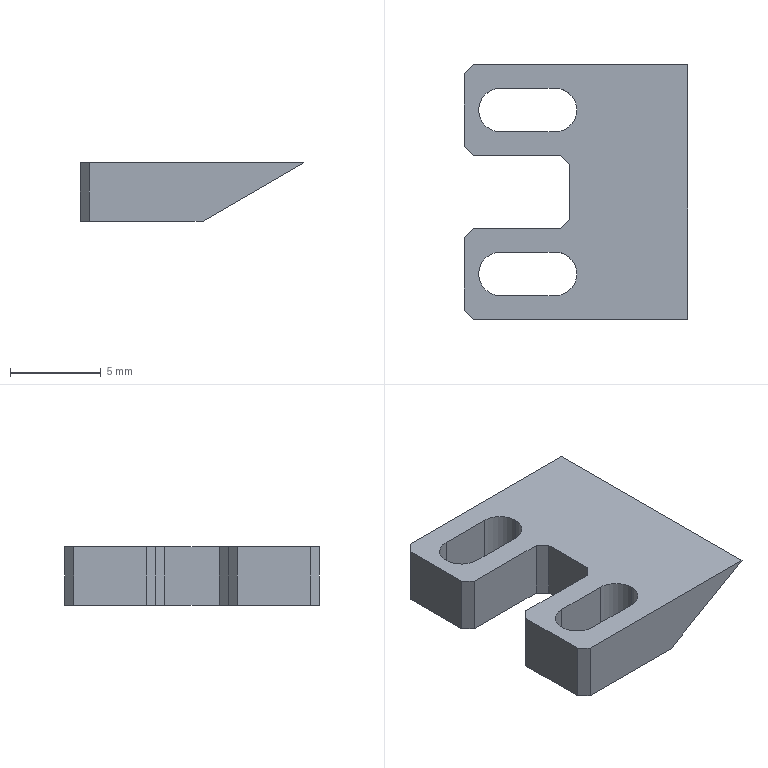Part | NX | 1 solid | 26 faces | box 12.3 x 14 x 3.2 mm | volume 276.814 mm3 | plane 20 | cylinder 6 | commonest cylinder face diameters 2.4 x6
STEP:
#1=CARTESIAN_POINT('',(0.05,4.5,-3.2));
#2=VERTEX_POINT('',#1);
#3=CARTESIAN_POINT('',(-1.15,5.7,-3.2));
#4=VERTEX_POINT('',#3);
#5=CARTESIAN_POINT('',(-1.15,4.5,-3.2));
#6=DIRECTION('',(0.,0.,1.));
#7=DIRECTION('',(1.,0.,0.));
#8=AXIS2_PLACEMENT_3D('',#5,#6,#7);
#9=CIRCLE('',#8,1.2);
#10=EDGE_CURVE('',#2,#4,#9,.T.);
#11=ORIENTED_EDGE('',*,*,#10,.F.);
#12=CARTESIAN_POINT('',(0.05,4.5,0.));
#13=VERTEX_POINT('',#12);
#14=CARTESIAN_POINT('',(0.05,4.5,-3.2));
#15=DIRECTION('',(0.,0.,1.));
#16=VECTOR('',#15,1000.);
#17=LINE('',#14,#16);
#18=EDGE_CURVE('',#2,#13,#17,.T.);
#19=ORIENTED_EDGE('',*,*,#18,.T.);
#20=CARTESIAN_POINT('',(-1.15,5.7,0.));
#21=VERTEX_POINT('',#20);
#22=CARTESIAN_POINT('',(-1.15,4.5,0.));
#23=DIRECTION('',(0.,0.,1.));
#24=DIRECTION('',(1.,0.,0.));
#25=AXIS2_PLACEMENT_3D('',#22,#23,#24);
#26=CIRCLE('',#25,1.2);
#27=EDGE_CURVE('',#13,#21,#26,.T.);
#28=ORIENTED_EDGE('',*,*,#27,.T.);
#29=CARTESIAN_POINT('',(-1.15,5.7,-3.2));
#30=DIRECTION('',(0.,0.,1.));
#31=VECTOR('',#30,1000.);
#32=LINE('',#29,#31);
#33=EDGE_CURVE('',#4,#21,#32,.T.);
#34=ORIENTED_EDGE('',*,*,#33,.F.);
#35=EDGE_LOOP('',(#11,#19,#28,#34));
#36=FACE_BOUND('',#35,.T.);
#37=CARTESIAN_POINT('',(-1.15,4.5,-3.2));
#38=DIRECTION('',(0.,0.,1.));
#39=DIRECTION('',(-1.,0.,0.));
#40=AXIS2_PLACEMENT_3D('',#37,#38,#39);
#41=CYLINDRICAL_SURFACE('',#40,1.2);
#42=ADVANCED_FACE('',(#36),#41,.F.);
#43=CARTESIAN_POINT('',(0.05,-4.5,-3.2));
#44=VERTEX_POINT('',#43);
#45=CARTESIAN_POINT('',(-1.15,-3.3,-3.2));
#46=VERTEX_POINT('',#45);
#47=CARTESIAN_POINT('',(-1.15,-4.5,-3.2));
#48=DIRECTION('',(0.,0.,1.));
#49=DIRECTION('',(-1.,0.,0.));
#50=AXIS2_PLACEMENT_3D('',#47,#48,#49);
#51=CIRCLE('',#50,1.2);
#52=EDGE_CURVE('',#44,#46,#51,.T.);
#53=ORIENTED_EDGE('',*,*,#52,.F.);
#54=CARTESIAN_POINT('',(0.05,-4.5,0.));
#55=VERTEX_POINT('',#54);
#56=CARTESIAN_POINT('',(0.05,-4.5,-3.2));
#57=DIRECTION('',(0.,0.,1.));
#58=VECTOR('',#57,1000.);
#59=LINE('',#56,#58);
#60=EDGE_CURVE('',#44,#55,#59,.T.);
#61=ORIENTED_EDGE('',*,*,#60,.T.);
#62=CARTESIAN_POINT('',(-1.15,-3.3,0.));
#63=VERTEX_POINT('',#62);
#64=CARTESIAN_POINT('',(-1.15,-4.5,0.));
#65=DIRECTION('',(0.,0.,1.));
#66=DIRECTION('',(-1.,0.,0.));
#67=AXIS2_PLACEMENT_3D('',#64,#65,#66);
#68=CIRCLE('',#67,1.2);
#69=EDGE_CURVE('',#55,#63,#68,.T.);
#70=ORIENTED_EDGE('',*,*,#69,.T.);
#71=CARTESIAN_POINT('',(-1.15,-3.3,-3.2));
#72=DIRECTION('',(0.,0.,1.));
#73=VECTOR('',#72,1000.);
#74=LINE('',#71,#73);
#75=EDGE_CURVE('',#46,#63,#74,.T.);
#76=ORIENTED_EDGE('',*,*,#75,.F.);
#77=EDGE_LOOP('',(#53,#61,#70,#76));
#78=FACE_BOUND('',#77,.T.);
#79=CARTESIAN_POINT('',(-1.15,-4.5,-3.2));
#80=DIRECTION('',(0.,0.,1.));
#81=DIRECTION('',(-1.,0.,0.));
#82=AXIS2_PLACEMENT_3D('',#79,#80,#81);
#83=CYLINDRICAL_SURFACE('',#82,1.2);
#84=ADVANCED_FACE('',(#78),#83,.F.);
#85=CARTESIAN_POINT('',(-6.15,6.5,-3.2));
#86=VERTEX_POINT('',#85);
#87=CARTESIAN_POINT('',(-6.15,2.5,-3.2));
#88=VERTEX_POINT('',#87);
#89=CARTESIAN_POINT('',(-6.15,7.,-3.2));
#90=DIRECTION('',(0.,-1.,0.));
#91=VECTOR('',#90,1000.);
#92=LINE('',#89,#91);
#93=EDGE_CURVE('',#86,#88,#92,.T.);
#94=ORIENTED_EDGE('',*,*,#93,.T.);
#95=CARTESIAN_POINT('',(-6.15,2.5,0.));
#96=VERTEX_POINT('',#95);
#97=CARTESIAN_POINT('',(-6.15,2.5,0.));
#98=DIRECTION('',(0.,0.,1.));
#99=VECTOR('',#98,1000.);
#100=LINE('',#97,#99);
#101=EDGE_CURVE('',#88,#96,#100,.T.);
#102=ORIENTED_EDGE('',*,*,#101,.T.);
#103=CARTESIAN_POINT('',(-6.15,6.5,0.));
#104=VERTEX_POINT('',#103);
#105=CARTESIAN_POINT('',(-6.15,7.,0.));
#106=DIRECTION('',(0.,-1.,0.));
#107=VECTOR('',#106,1000.);
#108=LINE('',#105,#107);
#109=EDGE_CURVE('',#104,#96,#108,.T.);
#110=ORIENTED_EDGE('',*,*,#109,.F.);
#111=CARTESIAN_POINT('',(-6.15,6.5,-3.2));
#112=DIRECTION('',(0.,0.,-1.));
#113=VECTOR('',#112,1000.);
#114=LINE('',#111,#113);
#115=EDGE_CURVE('',#104,#86,#114,.T.);
#116=ORIENTED_EDGE('',*,*,#115,.T.);
#117=EDGE_LOOP('',(#94,#102,#110,#116));
#118=FACE_BOUND('',#117,.T.);
#119=CARTESIAN_POINT('',(-6.15,7.,0.));
#120=DIRECTION('',(1.,0.,0.));
#121=DIRECTION('',(0.,-1.,0.));
#122=AXIS2_PLACEMENT_3D('',#119,#120,#121);
#123=PLANE('',#122);
#124=ADVANCED_FACE('',(#118),#123,.F.);
#125=CARTESIAN_POINT('',(6.15,-7.,0.));
#126=VERTEX_POINT('',#125);
#127=CARTESIAN_POINT('',(0.6074,-7.,-3.2));
#128=VERTEX_POINT('',#127);
#129=CARTESIAN_POINT('',(0.6074,-7.,-3.2));
#130=DIRECTION('',(-0.866,0.,-0.5));
#131=VECTOR('',#130,1000.);
#132=LINE('',#129,#131);
#133=EDGE_CURVE('',#126,#128,#132,.T.);
#134=ORIENTED_EDGE('',*,*,#133,.T.);
#135=CARTESIAN_POINT('',(0.6074,7.,-3.2));
#136=VERTEX_POINT('',#135);
#137=CARTESIAN_POINT('',(0.6074,7.,-3.2));
#138=DIRECTION('',(0.,-1.,0.));
#139=VECTOR('',#138,1000.);
#140=LINE('',#137,#139);
#141=EDGE_CURVE('',#136,#128,#140,.T.);
#142=ORIENTED_EDGE('',*,*,#141,.F.);
#143=CARTESIAN_POINT('',(6.15,7.,0.));
#144=VERTEX_POINT('',#143);
#145=CARTESIAN_POINT('',(0.6074,7.,-3.2));
#146=DIRECTION('',(-0.866,0.,-0.5));
#147=VECTOR('',#146,1000.);
#148=LINE('',#145,#147);
#149=EDGE_CURVE('',#144,#136,#148,.T.);
#150=ORIENTED_EDGE('',*,*,#149,.F.);
#151=CARTESIAN_POINT('',(6.15,7.,0.));
#152=DIRECTION('',(0.,-1.,0.));
#153=VECTOR('',#152,1000.);
#154=LINE('',#151,#153);
#155=EDGE_CURVE('',#144,#126,#154,.T.);
#156=ORIENTED_EDGE('',*,*,#155,.T.);
#157=EDGE_LOOP('',(#134,#142,#150,#156));
#158=FACE_BOUND('',#157,.T.);
#159=CARTESIAN_POINT('',(0.6074,7.,-3.2));
#160=DIRECTION('',(-0.5,0.,0.866));
#161=DIRECTION('',(-0.866,0.,-0.5));
#162=AXIS2_PLACEMENT_3D('',#159,#160,#161);
#163=PLANE('',#162);
#164=ADVANCED_FACE('',(#158),#163,.F.);
#165=CARTESIAN_POINT('',(-4.15,3.3,-3.2));
#166=VERTEX_POINT('',#165);
#167=CARTESIAN_POINT('',(-1.15,3.3,-3.2));
#168=VERTEX_POINT('',#167);
#169=CARTESIAN_POINT('',(-1.15,3.3,-3.2));
#170=DIRECTION('',(1.,0.,0.));
#171=VECTOR('',#170,1000.);
#172=LINE('',#169,#171);
#173=EDGE_CURVE('',#166,#168,#172,.T.);
#174=ORIENTED_EDGE('',*,*,#173,.T.);
#175=CARTESIAN_POINT('',(-1.15,4.5,-3.2));
#176=DIRECTION('',(0.,0.,1.));
#177=DIRECTION('',(1.,0.,0.));
#178=AXIS2_PLACEMENT_3D('',#175,#176,#177);
#179=CIRCLE('',#178,1.2);
#180=EDGE_CURVE('',#168,#2,#179,.T.);
#181=ORIENTED_EDGE('',*,*,#180,.T.);
#182=ORIENTED_EDGE('',*,*,#10,.T.);
#183=CARTESIAN_POINT('',(-4.15,5.7,-3.2));
#184=VERTEX_POINT('',#183);
#185=CARTESIAN_POINT('',(-1.15,5.7,-3.2));
#186=DIRECTION('',(-1.,0.,0.));
#187=VECTOR('',#186,1000.);
#188=LINE('',#185,#187);
#189=EDGE_CURVE('',#4,#184,#188,.T.);
#190=ORIENTED_EDGE('',*,*,#189,.T.);
#191=CARTESIAN_POINT('',(-4.15,4.5,-3.2));
#192=DIRECTION('',(0.,0.,1.));
#193=DIRECTION('',(1.,0.,0.));
#194=AXIS2_PLACEMENT_3D('',#191,#192,#193);
#195=CIRCLE('',#194,1.2);
#196=EDGE_CURVE('',#184,#166,#195,.T.);
#197=ORIENTED_EDGE('',*,*,#196,.T.);
#198=EDGE_LOOP('',(#174,#181,#182,#190,#197));
#199=FACE_BOUND('',#198,.T.);
#200=CARTESIAN_POINT('',(-4.15,-5.7,-3.2));
#201=VERTEX_POINT('',#200);
#202=CARTESIAN_POINT('',(-1.15,-5.7,-3.2));
#203=VERTEX_POINT('',#202);
#204=CARTESIAN_POINT('',(-1.15,-5.7,-3.2));
#205=DIRECTION('',(1.,0.,0.));
#206=VECTOR('',#205,1000.);
#207=LINE('',#204,#206);
#208=EDGE_CURVE('',#201,#203,#207,.T.);
#209=ORIENTED_EDGE('',*,*,#208,.T.);
#210=CARTESIAN_POINT('',(-1.15,-4.5,-3.2));
#211=DIRECTION('',(0.,0.,1.));
#212=DIRECTION('',(-1.,0.,0.));
#213=AXIS2_PLACEMENT_3D('',#210,#211,#212);
#214=CIRCLE('',#213,1.2);
#215=EDGE_CURVE('',#203,#44,#214,.T.);
#216=ORIENTED_EDGE('',*,*,#215,.T.);
#217=ORIENTED_EDGE('',*,*,#52,.T.);
#218=CARTESIAN_POINT('',(-4.15,-3.3,-3.2));
#219=VERTEX_POINT('',#218);
#220=CARTESIAN_POINT('',(-1.15,-3.3,-3.2));
#221=DIRECTION('',(-1.,0.,0.));
#222=VECTOR('',#221,1000.);
#223=LINE('',#220,#222);
#224=EDGE_CURVE('',#46,#219,#223,.T.);
#225=ORIENTED_EDGE('',*,*,#224,.T.);
#226=CARTESIAN_POINT('',(-4.15,-4.5,-3.2));
#227=DIRECTION('',(0.,0.,1.));
#228=DIRECTION('',(-1.,0.,0.));
#229=AXIS2_PLACEMENT_3D('',#226,#227,#228);
#230=CIRCLE('',#229,1.2);
#231=EDGE_CURVE('',#219,#201,#230,.T.);
#232=ORIENTED_EDGE('',*,*,#231,.T.);
#233=EDGE_LOOP('',(#209,#216,#217,#225,#232));
#234=FACE_BOUND('',#233,.T.);
#235=CARTESIAN_POINT('',(-5.65,-7.,-3.2));
#236=VERTEX_POINT('',#235);
#237=CARTESIAN_POINT('',(-6.15,-7.,-3.2));
#238=DIRECTION('',(-1.,0.,0.));
#239=VECTOR('',#238,1000.);
#240=LINE('',#237,#239);
#241=EDGE_CURVE('',#128,#236,#240,.T.);
#242=ORIENTED_EDGE('',*,*,#241,.T.);
#243=CARTESIAN_POINT('',(-6.15,-6.5,-3.2));
#244=VERTEX_POINT('',#243);
#245=CARTESIAN_POINT('',(-6.15,-6.5,-3.2));
#246=DIRECTION('',(-0.7071,0.7071,0.));
#247=VECTOR('',#246,1000.);
#248=LINE('',#245,#247);
#249=EDGE_CURVE('',#236,#244,#248,.T.);
#250=ORIENTED_EDGE('',*,*,#249,.T.);
#251=CARTESIAN_POINT('',(-6.15,-2.5,-3.2));
#252=VERTEX_POINT('',#251);
#253=CARTESIAN_POINT('',(-6.15,7.,-3.2));
#254=DIRECTION('',(0.,-1.,0.));
#255=VECTOR('',#254,1000.);
#256=LINE('',#253,#255);
#257=EDGE_CURVE('',#252,#244,#256,.T.);
#258=ORIENTED_EDGE('',*,*,#257,.F.);
#259=CARTESIAN_POINT('',(-5.65,-2.,-3.2));
#260=VERTEX_POINT('',#259);
#261=CARTESIAN_POINT('',(-5.65,-2.,-3.2));
#262=DIRECTION('',(0.7071,0.7071,0.));
#263=VECTOR('',#262,1000.);
#264=LINE('',#261,#263);
#265=EDGE_CURVE('',#252,#260,#264,.T.);
#266=ORIENTED_EDGE('',*,*,#265,.T.);
#267=CARTESIAN_POINT('',(-0.85,-2.,-3.2));
#268=VERTEX_POINT('',#267);
#269=CARTESIAN_POINT('',(-0.35,-2.,-3.2));
#270=DIRECTION('',(1.,0.,0.));
#271=VECTOR('',#270,1000.);
#272=LINE('',#269,#271);
#273=EDGE_CURVE('',#260,#268,#272,.T.);
#274=ORIENTED_EDGE('',*,*,#273,.T.);
#275=CARTESIAN_POINT('',(-0.35,-1.5,-3.2));
#276=VERTEX_POINT('',#275);
#277=CARTESIAN_POINT('',(1.,-0.15,-3.2));
#278=DIRECTION('',(0.7071,0.7071,0.));
#279=VECTOR('',#278,1000.);
#280=LINE('',#277,#279);
#281=EDGE_CURVE('',#268,#276,#280,.T.);
#282=ORIENTED_EDGE('',*,*,#281,.T.);
#283=CARTESIAN_POINT('',(-0.35,1.5,-3.2));
#284=VERTEX_POINT('',#283);
#285=CARTESIAN_POINT('',(-0.35,2.,-3.2));
#286=DIRECTION('',(0.,1.,0.));
#287=VECTOR('',#286,1000.);
#288=LINE('',#285,#287);
#289=EDGE_CURVE('',#276,#284,#288,.T.);
#290=ORIENTED_EDGE('',*,*,#289,.T.);
#291=CARTESIAN_POINT('',(-0.85,2.,-3.2));
#292=VERTEX_POINT('',#291);
#293=CARTESIAN_POINT('',(-6.,7.15,-3.2));
#294=DIRECTION('',(-0.7071,0.7071,0.));
#295=VECTOR('',#294,1000.);
#296=LINE('',#293,#295);
#297=EDGE_CURVE('',#284,#292,#296,.T.);
#298=ORIENTED_EDGE('',*,*,#297,.T.);
#299=CARTESIAN_POINT('',(-5.65,2.,-3.2));
#300=VERTEX_POINT('',#299);
#301=CARTESIAN_POINT('',(-6.15,2.,-3.2));
#302=DIRECTION('',(-1.,0.,0.));
#303=VECTOR('',#302,1000.);
#304=LINE('',#301,#303);
#305=EDGE_CURVE('',#292,#300,#304,.T.);
#306=ORIENTED_EDGE('',*,*,#305,.T.);
#307=CARTESIAN_POINT('',(-6.15,2.5,-3.2));
#308=DIRECTION('',(-0.7071,0.7071,0.));
#309=VECTOR('',#308,1000.);
#310=LINE('',#307,#309);
#311=EDGE_CURVE('',#300,#88,#310,.T.);
#312=ORIENTED_EDGE('',*,*,#311,.T.);
#313=ORIENTED_EDGE('',*,*,#93,.F.);
#314=CARTESIAN_POINT('',(-5.65,7.,-3.2));
#315=VERTEX_POINT('',#314);
#316=CARTESIAN_POINT('',(-5.65,7.,-3.2));
#317=DIRECTION('',(0.7071,0.7071,0.));
#318=VECTOR('',#317,1000.);
#319=LINE('',#316,#318);
#320=EDGE_CURVE('',#86,#315,#319,.T.);
#321=ORIENTED_EDGE('',*,*,#320,.T.);
#322=CARTESIAN_POINT('',(-6.15,7.,-3.2));
#323=DIRECTION('',(-1.,0.,0.));
#324=VECTOR('',#323,1000.);
#325=LINE('',#322,#324);
#326=EDGE_CURVE('',#136,#315,#325,.T.);
#327=ORIENTED_EDGE('',*,*,#326,.F.);
#328=ORIENTED_EDGE('',*,*,#141,.T.);
#329=EDGE_LOOP('',(#242,#250,#258,#266,#274,#282,#290,#298,#306,#312,#313,#321,#327,#328));
#330=FACE_BOUND('',#329,.T.);
#331=CARTESIAN_POINT('',(-6.15,7.,-3.2));
#332=DIRECTION('',(0.,0.,1.));
#333=DIRECTION('',(0.,1.,0.));
#334=AXIS2_PLACEMENT_3D('',#331,#332,#333);
#335=PLANE('',#334);
#336=ADVANCED_FACE('',(#199,#234,#330),#335,.F.);
#337=ORIENTED_EDGE('',*,*,#257,.T.);
#338=CARTESIAN_POINT('',(-6.15,-6.5,0.));
#339=VERTEX_POINT('',#338);
#340=CARTESIAN_POINT('',(-6.15,-6.5,0.));
#341=DIRECTION('',(0.,0.,1.));
#342=VECTOR('',#341,1000.);
#343=LINE('',#340,#342);
#344=EDGE_CURVE('',#244,#339,#343,.T.);
#345=ORIENTED_EDGE('',*,*,#344,.T.);
#346=CARTESIAN_POINT('',(-6.15,-2.5,0.));
#347=VERTEX_POINT('',#346);
#348=CARTESIAN_POINT('',(-6.15,7.,0.));
#349=DIRECTION('',(0.,-1.,0.));
#350=VECTOR('',#349,1000.);
#351=LINE('',#348,#350);
#352=EDGE_CURVE('',#347,#339,#351,.T.);
#353=ORIENTED_EDGE('',*,*,#352,.F.);
#354=CARTESIAN_POINT('',(-6.15,-2.5,0.));
#355=DIRECTION('',(0.,0.,-1.));
#356=VECTOR('',#355,1000.);
#357=LINE('',#354,#356);
#358=EDGE_CURVE('',#347,#252,#357,.T.);
#359=ORIENTED_EDGE('',*,*,#358,.T.);
#360=EDGE_LOOP('',(#337,#345,#353,#359));
#361=FACE_BOUND('',#360,.T.);
#362=CARTESIAN_POINT('',(-6.15,7.,0.));
#363=DIRECTION('',(1.,0.,0.));
#364=DIRECTION('',(0.,-1.,0.));
#365=AXIS2_PLACEMENT_3D('',#362,#363,#364);
#366=PLANE('',#365);
#367=ADVANCED_FACE('',(#361),#366,.F.);
#368=CARTESIAN_POINT('',(-4.15,5.7,0.));
#369=VERTEX_POINT('',#368);
#370=CARTESIAN_POINT('',(-1.15,5.7,0.));
#371=DIRECTION('',(-1.,0.,0.));
#372=VECTOR('',#371,1000.);
#373=LINE('',#370,#372);
#374=EDGE_CURVE('',#21,#369,#373,.T.);
#375=ORIENTED_EDGE('',*,*,#374,.F.);
#376=ORIENTED_EDGE('',*,*,#27,.F.);
#377=CARTESIAN_POINT('',(-1.15,3.3,0.));
#378=VERTEX_POINT('',#377);
#379=CARTESIAN_POINT('',(-1.15,4.5,0.));
#380=DIRECTION('',(0.,0.,1.));
#381=DIRECTION('',(1.,0.,0.));
#382=AXIS2_PLACEMENT_3D('',#379,#380,#381);
#383=CIRCLE('',#382,1.2);
#384=EDGE_CURVE('',#378,#13,#383,.T.);
#385=ORIENTED_EDGE('',*,*,#384,.F.);
#386=CARTESIAN_POINT('',(-4.15,3.3,0.));
#387=VERTEX_POINT('',#386);
#388=CARTESIAN_POINT('',(-1.15,3.3,0.));
#389=DIRECTION('',(1.,0.,0.));
#390=VECTOR('',#389,1000.);
#391=LINE('',#388,#390);
#392=EDGE_CURVE('',#387,#378,#391,.T.);
#393=ORIENTED_EDGE('',*,*,#392,.F.);
#394=CARTESIAN_POINT('',(-4.15,4.5,0.));
#395=DIRECTION('',(0.,0.,1.));
#396=DIRECTION('',(1.,0.,0.));
#397=AXIS2_PLACEMENT_3D('',#394,#395,#396);
#398=CIRCLE('',#397,1.2);
#399=EDGE_CURVE('',#369,#387,#398,.T.);
#400=ORIENTED_EDGE('',*,*,#399,.F.);
#401=EDGE_LOOP('',(#375,#376,#385,#393,#400));
#402=FACE_BOUND('',#401,.T.);
#403=CARTESIAN_POINT('',(-4.15,-3.3,0.));
#404=VERTEX_POINT('',#403);
#405=CARTESIAN_POINT('',(-1.15,-3.3,0.));
#406=DIRECTION('',(-1.,0.,0.));
#407=VECTOR('',#406,1000.);
#408=LINE('',#405,#407);
#409=EDGE_CURVE('',#63,#404,#408,.T.);
#410=ORIENTED_EDGE('',*,*,#409,.F.);
#411=ORIENTED_EDGE('',*,*,#69,.F.);
#412=CARTESIAN_POINT('',(-1.15,-5.7,0.));
#413=VERTEX_POINT('',#412);
#414=CARTESIAN_POINT('',(-1.15,-4.5,0.));
#415=DIRECTION('',(0.,0.,1.));
#416=DIRECTION('',(-1.,0.,0.));
#417=AXIS2_PLACEMENT_3D('',#414,#415,#416);
#418=CIRCLE('',#417,1.2);
#419=EDGE_CURVE('',#413,#55,#418,.T.);
#420=ORIENTED_EDGE('',*,*,#419,.F.);
#421=CARTESIAN_POINT('',(-4.15,-5.7,0.));
#422=VERTEX_POINT('',#421);
#423=CARTESIAN_POINT('',(-1.15,-5.7,0.));
#424=DIRECTION('',(1.,0.,0.));
#425=VECTOR('',#424,1000.);
#426=LINE('',#423,#425);
#427=EDGE_CURVE('',#422,#413,#426,.T.);
#428=ORIENTED_EDGE('',*,*,#427,.F.);
#429=CARTESIAN_POINT('',(-4.15,-4.5,0.));
#430=DIRECTION('',(0.,0.,1.));
#431=DIRECTION('',(-1.,0.,0.));
#432=AXIS2_PLACEMENT_3D('',#429,#430,#431);
#433=CIRCLE('',#432,1.2);
#434=EDGE_CURVE('',#404,#422,#433,.T.);
#435=ORIENTED_EDGE('',*,*,#434,.F.);
#436=EDGE_LOOP('',(#410,#411,#420,#428,#435));
#437=FACE_BOUND('',#436,.T.);
#438=ORIENTED_EDGE('',*,*,#352,.T.);
#439=CARTESIAN_POINT('',(-5.65,-7.,0.));
#440=VERTEX_POINT('',#439);
#441=CARTESIAN_POINT('',(-6.15,-6.5,0.));
#442=DIRECTION('',(0.7071,-0.7071,0.));
#443=VECTOR('',#442,1000.);
#444=LINE('',#441,#443);
#445=EDGE_CURVE('',#339,#440,#444,.T.);
#446=ORIENTED_EDGE('',*,*,#445,.T.);
#447=CARTESIAN_POINT('',(6.15,-7.,0.));
#448=DIRECTION('',(1.,0.,0.));
#449=VECTOR('',#448,1000.);
#450=LINE('',#447,#449);
#451=EDGE_CURVE('',#440,#126,#450,.T.);
#452=ORIENTED_EDGE('',*,*,#451,.T.);
#453=ORIENTED_EDGE('',*,*,#155,.F.);
#454=CARTESIAN_POINT('',(-5.65,7.,0.));
#455=VERTEX_POINT('',#454);
#456=CARTESIAN_POINT('',(6.15,7.,0.));
#457=DIRECTION('',(1.,0.,0.));
#458=VECTOR('',#457,1000.);
#459=LINE('',#456,#458);
#460=EDGE_CURVE('',#455,#144,#459,.T.);
#461=ORIENTED_EDGE('',*,*,#460,.F.);
#462=CARTESIAN_POINT('',(-5.65,7.,0.));
#463=DIRECTION('',(-0.7071,-0.7071,0.));
#464=VECTOR('',#463,1000.);
#465=LINE('',#462,#464);
#466=EDGE_CURVE('',#455,#104,#465,.T.);
#467=ORIENTED_EDGE('',*,*,#466,.T.);
#468=ORIENTED_EDGE('',*,*,#109,.T.);
#469=CARTESIAN_POINT('',(-5.65,2.,0.));
#470=VERTEX_POINT('',#469);
#471=CARTESIAN_POINT('',(-6.15,2.5,0.));
#472=DIRECTION('',(0.7071,-0.7071,0.));
#473=VECTOR('',#472,1000.);
#474=LINE('',#471,#473);
#475=EDGE_CURVE('',#96,#470,#474,.T.);
#476=ORIENTED_EDGE('',*,*,#475,.T.);
#477=CARTESIAN_POINT('',(-0.85,2.,0.));
#478=VERTEX_POINT('',#477);
#479=CARTESIAN_POINT('',(-6.15,2.,0.));
#480=DIRECTION('',(-1.,0.,0.));
#481=VECTOR('',#480,1000.);
#482=LINE('',#479,#481);
#483=EDGE_CURVE('',#478,#470,#482,.T.);
#484=ORIENTED_EDGE('',*,*,#483,.F.);
#485=CARTESIAN_POINT('',(-0.35,1.5,0.));
#486=VERTEX_POINT('',#485);
#487=CARTESIAN_POINT('',(0.15,1.,0.));
#488=DIRECTION('',(0.7071,-0.7071,0.));
#489=VECTOR('',#488,1000.);
#490=LINE('',#487,#489);
#491=EDGE_CURVE('',#478,#486,#490,.T.);
#492=ORIENTED_EDGE('',*,*,#491,.T.);
#493=CARTESIAN_POINT('',(-0.35,-1.5,0.));
#494=VERTEX_POINT('',#493);
#495=CARTESIAN_POINT('',(-0.35,2.,0.));
#496=DIRECTION('',(0.,1.,0.));
#497=VECTOR('',#496,1000.);
#498=LINE('',#495,#497);
#499=EDGE_CURVE('',#494,#486,#498,.T.);
#500=ORIENTED_EDGE('',*,*,#499,.F.);
#501=CARTESIAN_POINT('',(-0.85,-2.,0.));
#502=VERTEX_POINT('',#501);
#503=CARTESIAN_POINT('',(7.15,6.,0.));
#504=DIRECTION('',(-0.7071,-0.7071,0.));
#505=VECTOR('',#504,1000.);
#506=LINE('',#503,#505);
#507=EDGE_CURVE('',#494,#502,#506,.T.);
#508=ORIENTED_EDGE('',*,*,#507,.T.);
#509=CARTESIAN_POINT('',(-5.65,-2.,0.));
#510=VERTEX_POINT('',#509);
#511=CARTESIAN_POINT('',(-0.35,-2.,0.));
#512=DIRECTION('',(1.,0.,0.));
#513=VECTOR('',#512,1000.);
#514=LINE('',#511,#513);
#515=EDGE_CURVE('',#510,#502,#514,.T.);
#516=ORIENTED_EDGE('',*,*,#515,.F.);
#517=CARTESIAN_POINT('',(-5.65,-2.,0.));
#518=DIRECTION('',(-0.7071,-0.7071,0.));
#519=VECTOR('',#518,1000.);
#520=LINE('',#517,#519);
#521=EDGE_CURVE('',#510,#347,#520,.T.);
#522=ORIENTED_EDGE('',*,*,#521,.T.);
#523=EDGE_LOOP('',(#438,#446,#452,#453,#461,#467,#468,#476,#484,#492,#500,#508,#516,#522));
#524=FACE_BOUND('',#523,.T.);
#525=CARTESIAN_POINT('',(6.15,7.,0.));
#526=DIRECTION('',(0.,0.,-1.));
#527=DIRECTION('',(1.,0.,0.));
#528=AXIS2_PLACEMENT_3D('',#525,#526,#527);
#529=PLANE('',#528);
#530=ADVANCED_FACE('',(#402,#437,#524),#529,.F.);
#531=ORIENTED_EDGE('',*,*,#326,.T.);
#532=CARTESIAN_POINT('',(-5.65,7.,0.));
#533=DIRECTION('',(0.,0.,1.));
#534=VECTOR('',#533,1000.);
#535=LINE('',#532,#534);
#536=EDGE_CURVE('',#315,#455,#535,.T.);
#537=ORIENTED_EDGE('',*,*,#536,.T.);
#538=ORIENTED_EDGE('',*,*,#460,.T.);
#539=ORIENTED_EDGE('',*,*,#149,.T.);
#540=EDGE_LOOP('',(#531,#537,#538,#539));
#541=FACE_BOUND('',#540,.T.);
#542=CARTESIAN_POINT('',(6.15,7.,0.));
#543=DIRECTION('',(0.,1.,0.));
#544=DIRECTION('',(0.,0.,-1.));
#545=AXIS2_PLACEMENT_3D('',#542,#543,#544);
#546=PLANE('',#545);
#547=ADVANCED_FACE('',(#541),#546,.T.);
#548=ORIENTED_EDGE('',*,*,#451,.F.);
#549=CARTESIAN_POINT('',(-5.65,-7.,0.));
#550=DIRECTION('',(0.,0.,-1.));
#551=VECTOR('',#550,1000.);
#552=LINE('',#549,#551);
#553=EDGE_CURVE('',#440,#236,#552,.T.);
#554=ORIENTED_EDGE('',*,*,#553,.T.);
#555=ORIENTED_EDGE('',*,*,#241,.F.);
#556=ORIENTED_EDGE('',*,*,#133,.F.);
#557=EDGE_LOOP('',(#548,#554,#555,#556));
#558=FACE_BOUND('',#557,.T.);
#559=CARTESIAN_POINT('',(6.15,-7.,0.));
#560=DIRECTION('',(0.,1.,0.));
#561=DIRECTION('',(0.,0.,-1.));
#562=AXIS2_PLACEMENT_3D('',#559,#560,#561);
#563=PLANE('',#562);
#564=ADVANCED_FACE('',(#558),#563,.F.);
#565=ORIENTED_EDGE('',*,*,#305,.F.);
#566=CARTESIAN_POINT('',(-0.85,2.,0.));
#567=DIRECTION('',(0.,0.,1.));
#568=VECTOR('',#567,1000.);
#569=LINE('',#566,#568);
#570=EDGE_CURVE('',#292,#478,#569,.T.);
#571=ORIENTED_EDGE('',*,*,#570,.T.);
#572=ORIENTED_EDGE('',*,*,#483,.T.);
#573=CARTESIAN_POINT('',(-5.65,2.,-3.2));
#574=DIRECTION('',(0.,0.,-1.));
#575=VECTOR('',#574,1000.);
#576=LINE('',#573,#575);
#577=EDGE_CURVE('',#470,#300,#576,.T.);
#578=ORIENTED_EDGE('',*,*,#577,.T.);
#579=EDGE_LOOP('',(#565,#571,#572,#578));
#580=FACE_BOUND('',#579,.T.);
#581=CARTESIAN_POINT('',(-6.15,2.,-3.2));
#582=DIRECTION('',(0.,1.,0.));
#583=DIRECTION('',(0.,0.,-1.));
#584=AXIS2_PLACEMENT_3D('',#581,#582,#583);
#585=PLANE('',#584);
#586=ADVANCED_FACE('',(#580),#585,.F.);
#587=ORIENTED_EDGE('',*,*,#289,.F.);
#588=CARTESIAN_POINT('',(-0.35,-1.5,0.));
#589=DIRECTION('',(0.,0.,1.));
#590=VECTOR('',#589,1000.);
#591=LINE('',#588,#590);
#592=EDGE_CURVE('',#276,#494,#591,.T.);
#593=ORIENTED_EDGE('',*,*,#592,.T.);
#594=ORIENTED_EDGE('',*,*,#499,.T.);
#595=CARTESIAN_POINT('',(-0.35,1.5,-3.2));
#596=DIRECTION('',(0.,0.,-1.));
#597=VECTOR('',#596,1000.);
#598=LINE('',#595,#597);
#599=EDGE_CURVE('',#486,#284,#598,.T.);
#600=ORIENTED_EDGE('',*,*,#599,.T.);
#601=EDGE_LOOP('',(#587,#593,#594,#600));
#602=FACE_BOUND('',#601,.T.);
#603=CARTESIAN_POINT('',(-0.35,2.,-3.2));
#604=DIRECTION('',(1.,0.,0.));
#605=DIRECTION('',(0.,0.,1.));
#606=AXIS2_PLACEMENT_3D('',#603,#604,#605);
#607=PLANE('',#606);
#608=ADVANCED_FACE('',(#602),#607,.F.);
#609=ORIENTED_EDGE('',*,*,#515,.T.);
#610=CARTESIAN_POINT('',(-0.85,-2.,-3.2));
#611=DIRECTION('',(0.,0.,-1.));
#612=VECTOR('',#611,1000.);
#613=LINE('',#610,#612);
#614=EDGE_CURVE('',#502,#268,#613,.T.);
#615=ORIENTED_EDGE('',*,*,#614,.T.);
#616=ORIENTED_EDGE('',*,*,#273,.F.);
#617=CARTESIAN_POINT('',(-5.65,-2.,-3.2));
#618=DIRECTION('',(0.,0.,1.));
#619=VECTOR('',#618,1000.);
#620=LINE('',#617,#619);
#621=EDGE_CURVE('',#260,#510,#620,.T.);
#622=ORIENTED_EDGE('',*,*,#621,.T.);
#623=EDGE_LOOP('',(#609,#615,#616,#622));
#624=FACE_BOUND('',#623,.T.);
#625=CARTESIAN_POINT('',(-0.35,-2.,-3.2));
#626=DIRECTION('',(0.,-1.,0.));
#627=DIRECTION('',(0.,0.,1.));
#628=AXIS2_PLACEMENT_3D('',#625,#626,#627);
#629=PLANE('',#628);
#630=ADVANCED_FACE('',(#624),#629,.F.);
#631=ORIENTED_EDGE('',*,*,#60,.F.);
#632=ORIENTED_EDGE('',*,*,#215,.F.);
#633=CARTESIAN_POINT('',(-1.15,-5.7,-3.2));
#634=DIRECTION('',(0.,0.,1.));
#635=VECTOR('',#634,1000.);
#636=LINE('',#633,#635);
#637=EDGE_CURVE('',#203,#413,#636,.T.);
#638=ORIENTED_EDGE('',*,*,#637,.T.);
#639=ORIENTED_EDGE('',*,*,#419,.T.);
#640=EDGE_LOOP('',(#631,#632,#638,#639));
#641=FACE_BOUND('',#640,.T.);
#642=CARTESIAN_POINT('',(-1.15,-4.5,-3.2));
#643=DIRECTION('',(0.,0.,1.));
#644=DIRECTION('',(-1.,0.,0.));
#645=AXIS2_PLACEMENT_3D('',#642,#643,#644);
#646=CYLINDRICAL_SURFACE('',#645,1.2);
#647=ADVANCED_FACE('',(#641),#646,.F.);
#648=ORIENTED_EDGE('',*,*,#427,.T.);
#649=ORIENTED_EDGE('',*,*,#637,.F.);
#650=ORIENTED_EDGE('',*,*,#208,.F.);
#651=CARTESIAN_POINT('',(-4.15,-5.7,-3.2));
#652=DIRECTION('',(0.,0.,1.));
#653=VECTOR('',#652,1000.);
#654=LINE('',#651,#653);
#655=EDGE_CURVE('',#201,#422,#654,.T.);
#656=ORIENTED_EDGE('',*,*,#655,.T.);
#657=EDGE_LOOP('',(#648,#649,#650,#656));
#658=FACE_BOUND('',#657,.T.);
#659=CARTESIAN_POINT('',(-1.15,-5.7,-3.2));
#660=DIRECTION('',(0.,-1.,0.));
#661=DIRECTION('',(-1.,0.,0.));
#662=AXIS2_PLACEMENT_3D('',#659,#660,#661);
#663=PLANE('',#662);
#664=ADVANCED_FACE('',(#658),#663,.F.);
#665=ORIENTED_EDGE('',*,*,#434,.T.);
#666=ORIENTED_EDGE('',*,*,#655,.F.);
#667=ORIENTED_EDGE('',*,*,#231,.F.);
#668=CARTESIAN_POINT('',(-4.15,-3.3,-3.2));
#669=DIRECTION('',(0.,0.,1.));
#670=VECTOR('',#669,1000.);
#671=LINE('',#668,#670);
#672=EDGE_CURVE('',#219,#404,#671,.T.);
#673=ORIENTED_EDGE('',*,*,#672,.T.);
#674=EDGE_LOOP('',(#665,#666,#667,#673));
#675=FACE_BOUND('',#674,.T.);
#676=CARTESIAN_POINT('',(-4.15,-4.5,-3.2));
#677=DIRECTION('',(0.,0.,1.));
#678=DIRECTION('',(-1.,0.,0.));
#679=AXIS2_PLACEMENT_3D('',#676,#677,#678);
#680=CYLINDRICAL_SURFACE('',#679,1.2);
#681=ADVANCED_FACE('',(#675),#680,.F.);
#682=ORIENTED_EDGE('',*,*,#409,.T.);
#683=ORIENTED_EDGE('',*,*,#672,.F.);
#684=ORIENTED_EDGE('',*,*,#224,.F.);
#685=ORIENTED_EDGE('',*,*,#75,.T.);
#686=EDGE_LOOP('',(#682,#683,#684,#685));
#687=FACE_BOUND('',#686,.T.);
#688=CARTESIAN_POINT('',(-1.15,-3.3,-3.2));
#689=DIRECTION('',(0.,1.,0.));
#690=DIRECTION('',(1.,0.,0.));
#691=AXIS2_PLACEMENT_3D('',#688,#689,#690);
#692=PLANE('',#691);
#693=ADVANCED_FACE('',(#687),#692,.F.);
#694=ORIENTED_EDGE('',*,*,#18,.F.);
#695=ORIENTED_EDGE('',*,*,#180,.F.);
#696=CARTESIAN_POINT('',(-1.15,3.3,-3.2));
#697=DIRECTION('',(0.,0.,1.));
#698=VECTOR('',#697,1000.);
#699=LINE('',#696,#698);
#700=EDGE_CURVE('',#168,#378,#699,.T.);
#701=ORIENTED_EDGE('',*,*,#700,.T.);
#702=ORIENTED_EDGE('',*,*,#384,.T.);
#703=EDGE_LOOP('',(#694,#695,#701,#702));
#704=FACE_BOUND('',#703,.T.);
#705=CARTESIAN_POINT('',(-1.15,4.5,-3.2));
#706=DIRECTION('',(0.,0.,1.));
#707=DIRECTION('',(-1.,0.,0.));
#708=AXIS2_PLACEMENT_3D('',#705,#706,#707);
#709=CYLINDRICAL_SURFACE('',#708,1.2);
#710=ADVANCED_FACE('',(#704),#709,.F.);
#711=ORIENTED_EDGE('',*,*,#392,.T.);
#712=ORIENTED_EDGE('',*,*,#700,.F.);
#713=ORIENTED_EDGE('',*,*,#173,.F.);
#714=CARTESIAN_POINT('',(-4.15,3.3,-3.2));
#715=DIRECTION('',(0.,0.,1.));
#716=VECTOR('',#715,1000.);
#717=LINE('',#714,#716);
#718=EDGE_CURVE('',#166,#387,#717,.T.);
#719=ORIENTED_EDGE('',*,*,#718,.T.);
#720=EDGE_LOOP('',(#711,#712,#713,#719));
#721=FACE_BOUND('',#720,.T.);
#722=CARTESIAN_POINT('',(-1.15,3.3,-3.2));
#723=DIRECTION('',(0.,-1.,0.));
#724=DIRECTION('',(0.,0.,1.));
#725=AXIS2_PLACEMENT_3D('',#722,#723,#724);
#726=PLANE('',#725);
#727=ADVANCED_FACE('',(#721),#726,.F.);
#728=ORIENTED_EDGE('',*,*,#399,.T.);
#729=ORIENTED_EDGE('',*,*,#718,.F.);
#730=ORIENTED_EDGE('',*,*,#196,.F.);
#731=CARTESIAN_POINT('',(-4.15,5.7,-3.2));
#732=DIRECTION('',(0.,0.,1.));
#733=VECTOR('',#732,1000.);
#734=LINE('',#731,#733);
#735=EDGE_CURVE('',#184,#369,#734,.T.);
#736=ORIENTED_EDGE('',*,*,#735,.T.);
#737=EDGE_LOOP('',(#728,#729,#730,#736));
#738=FACE_BOUND('',#737,.T.);
#739=CARTESIAN_POINT('',(-4.15,4.5,-3.2));
#740=DIRECTION('',(0.,0.,1.));
#741=DIRECTION('',(-1.,0.,0.));
#742=AXIS2_PLACEMENT_3D('',#739,#740,#741);
#743=CYLINDRICAL_SURFACE('',#742,1.2);
#744=ADVANCED_FACE('',(#738),#743,.F.);
#745=ORIENTED_EDGE('',*,*,#374,.T.);
#746=ORIENTED_EDGE('',*,*,#735,.F.);
#747=ORIENTED_EDGE('',*,*,#189,.F.);
#748=ORIENTED_EDGE('',*,*,#33,.T.);
#749=EDGE_LOOP('',(#745,#746,#747,#748));
#750=FACE_BOUND('',#749,.T.);
#751=CARTESIAN_POINT('',(-1.15,5.7,-3.2));
#752=DIRECTION('',(0.,1.,0.));
#753=DIRECTION('',(0.,0.,-1.));
#754=AXIS2_PLACEMENT_3D('',#751,#752,#753);
#755=PLANE('',#754);
#756=ADVANCED_FACE('',(#750),#755,.F.);
#757=ORIENTED_EDGE('',*,*,#281,.F.);
#758=ORIENTED_EDGE('',*,*,#614,.F.);
#759=ORIENTED_EDGE('',*,*,#507,.F.);
#760=ORIENTED_EDGE('',*,*,#592,.F.);
#761=EDGE_LOOP('',(#757,#758,#759,#760));
#762=FACE_BOUND('',#761,.T.);
#763=CARTESIAN_POINT('',(-0.35,-1.5,-3.2));
#764=DIRECTION('',(-0.7071,0.7071,0.));
#765=DIRECTION('',(0.,0.,1.));
#766=AXIS2_PLACEMENT_3D('',#763,#764,#765);
#767=PLANE('',#766);
#768=ADVANCED_FACE('',(#762),#767,.T.);
#769=ORIENTED_EDGE('',*,*,#297,.F.);
#770=ORIENTED_EDGE('',*,*,#599,.F.);
#771=ORIENTED_EDGE('',*,*,#491,.F.);
#772=ORIENTED_EDGE('',*,*,#570,.F.);
#773=EDGE_LOOP('',(#769,#770,#771,#772));
#774=FACE_BOUND('',#773,.T.);
#775=CARTESIAN_POINT('',(-0.85,2.,-3.2));
#776=DIRECTION('',(-0.7071,-0.7071,0.));
#777=DIRECTION('',(0.,0.,1.));
#778=AXIS2_PLACEMENT_3D('',#775,#776,#777);
#779=PLANE('',#778);
#780=ADVANCED_FACE('',(#774),#779,.T.);
#781=ORIENTED_EDGE('',*,*,#249,.F.);
#782=ORIENTED_EDGE('',*,*,#553,.F.);
#783=ORIENTED_EDGE('',*,*,#445,.F.);
#784=ORIENTED_EDGE('',*,*,#344,.F.);
#785=EDGE_LOOP('',(#781,#782,#783,#784));
#786=FACE_BOUND('',#785,.T.);
#787=CARTESIAN_POINT('',(-6.15,-6.5,0.));
#788=DIRECTION('',(0.7071,0.7071,0.));
#789=DIRECTION('',(0.,0.,-1.));
#790=AXIS2_PLACEMENT_3D('',#787,#788,#789);
#791=PLANE('',#790);
#792=ADVANCED_FACE('',(#786),#791,.F.);
#793=ORIENTED_EDGE('',*,*,#265,.F.);
#794=ORIENTED_EDGE('',*,*,#358,.F.);
#795=ORIENTED_EDGE('',*,*,#521,.F.);
#796=ORIENTED_EDGE('',*,*,#621,.F.);
#797=EDGE_LOOP('',(#793,#794,#795,#796));
#798=FACE_BOUND('',#797,.T.);
#799=CARTESIAN_POINT('',(-5.65,-2.,-3.2));
#800=DIRECTION('',(0.7071,-0.7071,0.));
#801=DIRECTION('',(0.,0.,-1.));
#802=AXIS2_PLACEMENT_3D('',#799,#800,#801);
#803=PLANE('',#802);
#804=ADVANCED_FACE('',(#798),#803,.F.);
#805=ORIENTED_EDGE('',*,*,#311,.F.);
#806=ORIENTED_EDGE('',*,*,#577,.F.);
#807=ORIENTED_EDGE('',*,*,#475,.F.);
#808=ORIENTED_EDGE('',*,*,#101,.F.);
#809=EDGE_LOOP('',(#805,#806,#807,#808));
#810=FACE_BOUND('',#809,.T.);
#811=CARTESIAN_POINT('',(-6.15,2.5,0.));
#812=DIRECTION('',(0.7071,0.7071,0.));
#813=DIRECTION('',(0.,0.,-1.));
#814=AXIS2_PLACEMENT_3D('',#811,#812,#813);
#815=PLANE('',#814);
#816=ADVANCED_FACE('',(#810),#815,.F.);
#817=ORIENTED_EDGE('',*,*,#320,.F.);
#818=ORIENTED_EDGE('',*,*,#115,.F.);
#819=ORIENTED_EDGE('',*,*,#466,.F.);
#820=ORIENTED_EDGE('',*,*,#536,.F.);
#821=EDGE_LOOP('',(#817,#818,#819,#820));
#822=FACE_BOUND('',#821,.T.);
#823=CARTESIAN_POINT('',(-5.65,7.,0.));
#824=DIRECTION('',(-0.7071,0.7071,0.));
#825=DIRECTION('',(0.,0.,1.));
#826=AXIS2_PLACEMENT_3D('',#823,#824,#825);
#827=PLANE('',#826);
#828=ADVANCED_FACE('',(#822),#827,.T.);
#829=CLOSED_SHELL('',(#42,#84,#124,#164,#336,#367,#530,#547,#564,#586,#608,#630,#647,#664,#681,#693,#710,#727,#744,#756,#768,#780,#792,#804,#816,#828));
#830=MANIFOLD_SOLID_BREP('',#829);
#831=(LENGTH_UNIT()NAMED_UNIT(*)SI_UNIT(.MILLI.,.METRE.));
#832=UNCERTAINTY_MEASURE_WITH_UNIT(LENGTH_MEASURE(0.00001),#831,'','');
#833=(NAMED_UNIT(*)PLANE_ANGLE_UNIT()SI_UNIT($,.RADIAN.));
#834=(NAMED_UNIT(*)SI_UNIT($,.STERADIAN.)SOLID_ANGLE_UNIT());
#835=(GEOMETRIC_REPRESENTATION_CONTEXT(3)GLOBAL_UNCERTAINTY_ASSIGNED_CONTEXT((#832))GLOBAL_UNIT_ASSIGNED_CONTEXT((#831,#833,#834))REPRESENTATION_CONTEXT('',''));
#836=ADVANCED_BREP_SHAPE_REPRESENTATION('',(#830),#835);